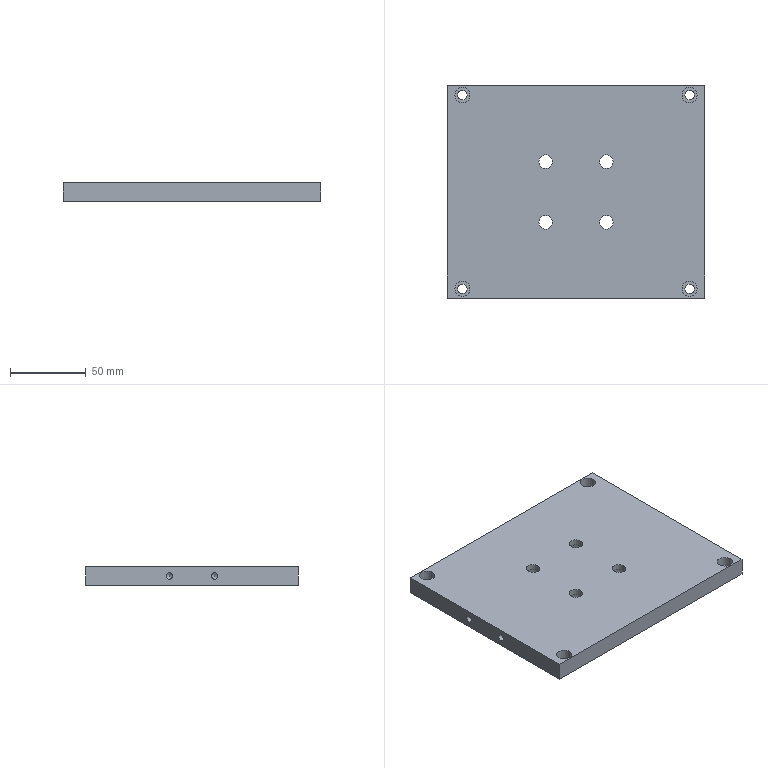Part | STEP file | 1 solid | 34 faces | box 170 x 140 x 12 mm | volume 277063 mm3 | cylinder 18 | plane 14 | cone 2 | commonest cylinder face diameters 6.2 x4 9 x4 10 x4 13 x4 4.2 x2